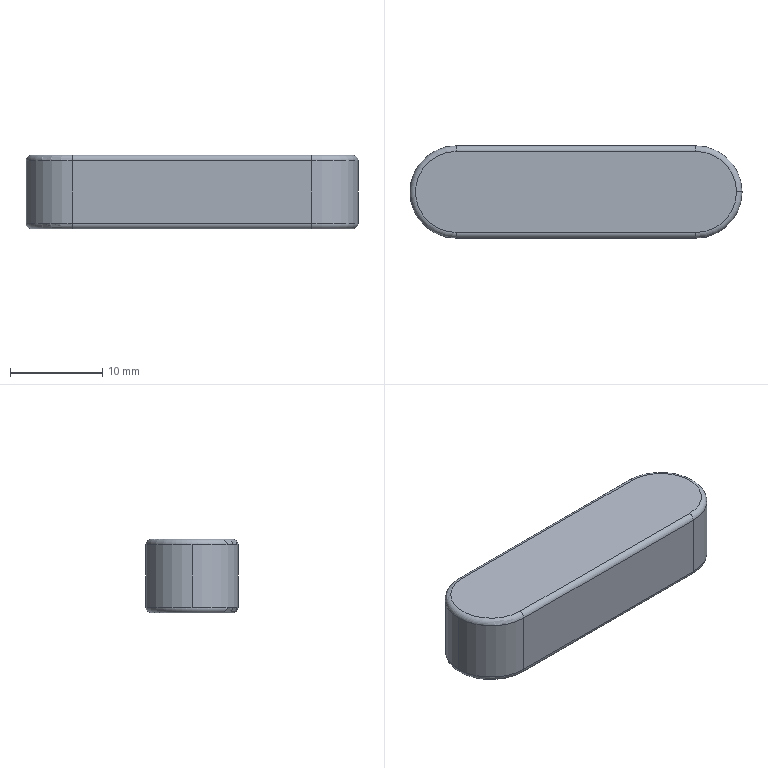Part | SolidWorks | features Extrusion 1, Fillet 1 | 1 solid | 17 faces | box 36 x 10 x 8 mm | volume 2696 mm3 | cylinder 7 | torus 6 | plane 4 | commonest cylinder face diameters 1.2 x4 10 x3
STEP:
#1=CARTESIAN_POINT('',(17.4,0.,0.));
#2=VERTEX_POINT('',#1);
#3=CARTESIAN_POINT('',(13.,-4.4,0.));
#4=VERTEX_POINT('',#3);
#5=CARTESIAN_POINT('',(13.,0.,0.));
#6=DIRECTION('',(0.,0.,-1.));
#7=DIRECTION('',(1.,0.,0.));
#8=AXIS2_PLACEMENT_3D('',#5,#6,#7);
#9=CIRCLE('',#8,4.4);
#10=EDGE_CURVE('',#2,#4,#9,.T.);
#11=ORIENTED_EDGE('',*,*,#10,.F.);
#12=CARTESIAN_POINT('',(18.,0.,0.6));
#13=VERTEX_POINT('',#12);
#14=CARTESIAN_POINT('',(17.4,0.,0.6));
#15=DIRECTION('',(0.,-1.,0.));
#16=DIRECTION('',(0.,0.,-1.));
#17=AXIS2_PLACEMENT_3D('',#14,#15,#16);
#18=CIRCLE('',#17,0.6);
#19=EDGE_CURVE('',#2,#13,#18,.T.);
#20=ORIENTED_EDGE('',*,*,#19,.T.);
#21=CARTESIAN_POINT('',(13.,-5.,0.6));
#22=VERTEX_POINT('',#21);
#23=CARTESIAN_POINT('',(13.,0.,0.6));
#24=DIRECTION('',(0.,0.,1.));
#25=DIRECTION('',(1.,0.,0.));
#26=AXIS2_PLACEMENT_3D('',#23,#24,#25);
#27=CIRCLE('',#26,5.);
#28=EDGE_CURVE('',#22,#13,#27,.T.);
#29=ORIENTED_EDGE('',*,*,#28,.F.);
#30=CARTESIAN_POINT('',(13.,-4.4,0.6));
#31=DIRECTION('',(1.,0.,0.));
#32=DIRECTION('',(0.,0.,-1.));
#33=AXIS2_PLACEMENT_3D('',#30,#31,#32);
#34=CIRCLE('',#33,0.6);
#35=EDGE_CURVE('',#22,#4,#34,.T.);
#36=ORIENTED_EDGE('',*,*,#35,.T.);
#37=EDGE_LOOP('',(#11,#20,#29,#36));
#38=FACE_OUTER_BOUND('',#37,.T.);
#39=CARTESIAN_POINT('',(13.,0.,0.6));
#40=DIRECTION('',(0.,0.,1.));
#41=DIRECTION('',(1.,0.,0.));
#42=AXIS2_PLACEMENT_3D('',#39,#40,#41);
#43=TOROIDAL_SURFACE('',#42,4.4,0.6);
#44=ADVANCED_FACE('',(#38),#43,.T.);
#45=CARTESIAN_POINT('',(18.,0.,7.4));
#46=VERTEX_POINT('',#45);
#47=CARTESIAN_POINT('',(13.,-5.,7.4));
#48=VERTEX_POINT('',#47);
#49=CARTESIAN_POINT('',(13.,0.,7.4));
#50=DIRECTION('',(0.,0.,-1.));
#51=DIRECTION('',(1.,0.,0.));
#52=AXIS2_PLACEMENT_3D('',#49,#50,#51);
#53=CIRCLE('',#52,5.);
#54=EDGE_CURVE('',#46,#48,#53,.T.);
#55=ORIENTED_EDGE('',*,*,#54,.F.);
#56=CARTESIAN_POINT('',(17.4,0.,8.));
#57=VERTEX_POINT('',#56);
#58=CARTESIAN_POINT('',(17.4,0.,7.4));
#59=DIRECTION('',(0.,-1.,0.));
#60=DIRECTION('',(0.,0.,-1.));
#61=AXIS2_PLACEMENT_3D('',#58,#59,#60);
#62=CIRCLE('',#61,0.6);
#63=EDGE_CURVE('',#46,#57,#62,.T.);
#64=ORIENTED_EDGE('',*,*,#63,.T.);
#65=CARTESIAN_POINT('',(13.,-4.4,8.));
#66=VERTEX_POINT('',#65);
#67=CARTESIAN_POINT('',(13.,0.,8.));
#68=DIRECTION('',(0.,0.,1.));
#69=DIRECTION('',(1.,0.,0.));
#70=AXIS2_PLACEMENT_3D('',#67,#68,#69);
#71=CIRCLE('',#70,4.4);
#72=EDGE_CURVE('',#66,#57,#71,.T.);
#73=ORIENTED_EDGE('',*,*,#72,.F.);
#74=CARTESIAN_POINT('',(13.,-4.4,7.4));
#75=DIRECTION('',(1.,0.,0.));
#76=DIRECTION('',(0.,0.,-1.));
#77=AXIS2_PLACEMENT_3D('',#74,#75,#76);
#78=CIRCLE('',#77,0.6);
#79=EDGE_CURVE('',#66,#48,#78,.T.);
#80=ORIENTED_EDGE('',*,*,#79,.T.);
#81=EDGE_LOOP('',(#55,#64,#73,#80));
#82=FACE_OUTER_BOUND('',#81,.T.);
#83=CARTESIAN_POINT('',(13.,0.,7.4));
#84=DIRECTION('',(0.,0.,1.));
#85=DIRECTION('',(1.,0.,0.));
#86=AXIS2_PLACEMENT_3D('',#83,#84,#85);
#87=TOROIDAL_SURFACE('',#86,4.4,0.6);
#88=ADVANCED_FACE('',(#82),#87,.T.);
#89=CARTESIAN_POINT('',(-13.,-5.,7.4));
#90=VERTEX_POINT('',#89);
#91=CARTESIAN_POINT('',(-18.,0.,7.4));
#92=VERTEX_POINT('',#91);
#93=CARTESIAN_POINT('',(-13.,0.,7.4));
#94=DIRECTION('',(0.,0.,-1.));
#95=DIRECTION('',(1.,0.,0.));
#96=AXIS2_PLACEMENT_3D('',#93,#94,#95);
#97=CIRCLE('',#96,5.);
#98=EDGE_CURVE('',#90,#92,#97,.T.);
#99=ORIENTED_EDGE('',*,*,#98,.T.);
#100=CARTESIAN_POINT('',(-18.,0.,0.6));
#101=VERTEX_POINT('',#100);
#102=CARTESIAN_POINT('',(-18.,0.,8.));
#103=DIRECTION('',(0.,0.,-1.));
#104=VECTOR('',#103,1000.);
#105=LINE('',#102,#104);
#106=EDGE_CURVE('',#92,#101,#105,.T.);
#107=ORIENTED_EDGE('',*,*,#106,.T.);
#108=CARTESIAN_POINT('',(-13.,-5.,0.6));
#109=VERTEX_POINT('',#108);
#110=CARTESIAN_POINT('',(-13.,0.,0.6));
#111=DIRECTION('',(0.,0.,1.));
#112=DIRECTION('',(1.,0.,0.));
#113=AXIS2_PLACEMENT_3D('',#110,#111,#112);
#114=CIRCLE('',#113,5.);
#115=EDGE_CURVE('',#101,#109,#114,.T.);
#116=ORIENTED_EDGE('',*,*,#115,.T.);
#117=CARTESIAN_POINT('',(-13.,-5.,8.));
#118=DIRECTION('',(0.,0.,-1.));
#119=VECTOR('',#118,1000.);
#120=LINE('',#117,#119);
#121=EDGE_CURVE('',#90,#109,#120,.T.);
#122=ORIENTED_EDGE('',*,*,#121,.F.);
#123=EDGE_LOOP('',(#99,#107,#116,#122));
#124=FACE_OUTER_BOUND('',#123,.T.);
#125=CARTESIAN_POINT('',(-13.,0.,8.));
#126=DIRECTION('',(0.,0.,-1.));
#127=DIRECTION('',(-1.,0.,0.));
#128=AXIS2_PLACEMENT_3D('',#125,#126,#127);
#129=CYLINDRICAL_SURFACE('',#128,5.);
#130=ADVANCED_FACE('',(#124),#129,.T.);
#131=ORIENTED_EDGE('',*,*,#106,.F.);
#132=CARTESIAN_POINT('',(-13.,5.,7.4));
#133=VERTEX_POINT('',#132);
#134=CARTESIAN_POINT('',(-13.,0.,7.4));
#135=DIRECTION('',(0.,0.,-1.));
#136=DIRECTION('',(1.,0.,0.));
#137=AXIS2_PLACEMENT_3D('',#134,#135,#136);
#138=CIRCLE('',#137,5.);
#139=EDGE_CURVE('',#92,#133,#138,.T.);
#140=ORIENTED_EDGE('',*,*,#139,.T.);
#141=CARTESIAN_POINT('',(-13.,5.,0.6));
#142=VERTEX_POINT('',#141);
#143=CARTESIAN_POINT('',(-13.,5.,8.));
#144=DIRECTION('',(0.,0.,-1.));
#145=VECTOR('',#144,1000.);
#146=LINE('',#143,#145);
#147=EDGE_CURVE('',#133,#142,#146,.T.);
#148=ORIENTED_EDGE('',*,*,#147,.T.);
#149=CARTESIAN_POINT('',(-13.,0.,0.6));
#150=DIRECTION('',(0.,0.,1.));
#151=DIRECTION('',(1.,0.,0.));
#152=AXIS2_PLACEMENT_3D('',#149,#150,#151);
#153=CIRCLE('',#152,5.);
#154=EDGE_CURVE('',#142,#101,#153,.T.);
#155=ORIENTED_EDGE('',*,*,#154,.T.);
#156=EDGE_LOOP('',(#131,#140,#148,#155));
#157=FACE_OUTER_BOUND('',#156,.T.);
#158=CARTESIAN_POINT('',(-13.,0.,8.));
#159=DIRECTION('',(0.,0.,-1.));
#160=DIRECTION('',(-1.,0.,0.));
#161=AXIS2_PLACEMENT_3D('',#158,#159,#160);
#162=CYLINDRICAL_SURFACE('',#161,5.);
#163=ADVANCED_FACE('',(#157),#162,.T.);
#164=CARTESIAN_POINT('',(13.,-5.,8.));
#165=DIRECTION('',(0.,0.,-1.));
#166=VECTOR('',#165,1000.);
#167=LINE('',#164,#166);
#168=EDGE_CURVE('',#48,#22,#167,.T.);
#169=ORIENTED_EDGE('',*,*,#168,.F.);
#170=CARTESIAN_POINT('',(-13.,-5.,7.4));
#171=DIRECTION('',(-1.,0.,0.));
#172=VECTOR('',#171,1000.);
#173=LINE('',#170,#172);
#174=EDGE_CURVE('',#48,#90,#173,.T.);
#175=ORIENTED_EDGE('',*,*,#174,.T.);
#176=ORIENTED_EDGE('',*,*,#121,.T.);
#177=CARTESIAN_POINT('',(-13.,-5.,0.6));
#178=DIRECTION('',(1.,0.,0.));
#179=VECTOR('',#178,1000.);
#180=LINE('',#177,#179);
#181=EDGE_CURVE('',#109,#22,#180,.T.);
#182=ORIENTED_EDGE('',*,*,#181,.T.);
#183=EDGE_LOOP('',(#169,#175,#176,#182));
#184=FACE_OUTER_BOUND('',#183,.T.);
#185=CARTESIAN_POINT('',(-13.,-5.,8.));
#186=DIRECTION('',(0.,1.,0.));
#187=DIRECTION('',(-1.,0.,0.));
#188=AXIS2_PLACEMENT_3D('',#185,#186,#187);
#189=PLANE('',#188);
#190=ADVANCED_FACE('',(#184),#189,.F.);
#191=CARTESIAN_POINT('',(13.,5.,7.4));
#192=VERTEX_POINT('',#191);
#193=CARTESIAN_POINT('',(13.,5.,0.6));
#194=VERTEX_POINT('',#193);
#195=CARTESIAN_POINT('',(13.,5.,8.));
#196=DIRECTION('',(0.,0.,-1.));
#197=VECTOR('',#196,1000.);
#198=LINE('',#195,#197);
#199=EDGE_CURVE('',#192,#194,#198,.T.);
#200=ORIENTED_EDGE('',*,*,#199,.F.);
#201=CARTESIAN_POINT('',(13.,0.,7.4));
#202=DIRECTION('',(0.,0.,-1.));
#203=DIRECTION('',(1.,0.,0.));
#204=AXIS2_PLACEMENT_3D('',#201,#202,#203);
#205=CIRCLE('',#204,5.);
#206=EDGE_CURVE('',#192,#46,#205,.T.);
#207=ORIENTED_EDGE('',*,*,#206,.T.);
#208=ORIENTED_EDGE('',*,*,#54,.T.);
#209=ORIENTED_EDGE('',*,*,#168,.T.);
#210=ORIENTED_EDGE('',*,*,#28,.T.);
#211=CARTESIAN_POINT('',(13.,0.,0.6));
#212=DIRECTION('',(0.,0.,1.));
#213=DIRECTION('',(1.,0.,0.));
#214=AXIS2_PLACEMENT_3D('',#211,#212,#213);
#215=CIRCLE('',#214,5.);
#216=EDGE_CURVE('',#13,#194,#215,.T.);
#217=ORIENTED_EDGE('',*,*,#216,.T.);
#218=EDGE_LOOP('',(#200,#207,#208,#209,#210,#217));
#219=FACE_OUTER_BOUND('',#218,.T.);
#220=CARTESIAN_POINT('',(13.,0.,8.));
#221=DIRECTION('',(0.,0.,-1.));
#222=DIRECTION('',(-1.,0.,0.));
#223=AXIS2_PLACEMENT_3D('',#220,#221,#222);
#224=CYLINDRICAL_SURFACE('',#223,5.);
#225=ADVANCED_FACE('',(#219),#224,.T.);
#226=ORIENTED_EDGE('',*,*,#147,.F.);
#227=CARTESIAN_POINT('',(13.,5.,7.4));
#228=DIRECTION('',(1.,0.,0.));
#229=VECTOR('',#228,1000.);
#230=LINE('',#227,#229);
#231=EDGE_CURVE('',#133,#192,#230,.T.);
#232=ORIENTED_EDGE('',*,*,#231,.T.);
#233=ORIENTED_EDGE('',*,*,#199,.T.);
#234=CARTESIAN_POINT('',(-13.,5.,0.6));
#235=DIRECTION('',(-1.,0.,0.));
#236=VECTOR('',#235,1000.);
#237=LINE('',#234,#236);
#238=EDGE_CURVE('',#194,#142,#237,.T.);
#239=ORIENTED_EDGE('',*,*,#238,.T.);
#240=EDGE_LOOP('',(#226,#232,#233,#239));
#241=FACE_OUTER_BOUND('',#240,.T.);
#242=CARTESIAN_POINT('',(-13.,5.,8.));
#243=DIRECTION('',(0.,-1.,0.));
#244=DIRECTION('',(1.,0.,0.));
#245=AXIS2_PLACEMENT_3D('',#242,#243,#244);
#246=PLANE('',#245);
#247=ADVANCED_FACE('',(#241),#246,.F.);
#248=CARTESIAN_POINT('',(-13.,-4.4,8.));
#249=VERTEX_POINT('',#248);
#250=CARTESIAN_POINT('',(13.,-4.4,8.));
#251=DIRECTION('',(1.,0.,0.));
#252=VECTOR('',#251,1000.);
#253=LINE('',#250,#252);
#254=EDGE_CURVE('',#249,#66,#253,.T.);
#255=ORIENTED_EDGE('',*,*,#254,.T.);
#256=ORIENTED_EDGE('',*,*,#72,.T.);
#257=CARTESIAN_POINT('',(13.,4.4,8.));
#258=VERTEX_POINT('',#257);
#259=CARTESIAN_POINT('',(13.,0.,8.));
#260=DIRECTION('',(0.,0.,1.));
#261=DIRECTION('',(1.,0.,0.));
#262=AXIS2_PLACEMENT_3D('',#259,#260,#261);
#263=CIRCLE('',#262,4.4);
#264=EDGE_CURVE('',#57,#258,#263,.T.);
#265=ORIENTED_EDGE('',*,*,#264,.T.);
#266=CARTESIAN_POINT('',(-13.,4.4,8.));
#267=VERTEX_POINT('',#266);
#268=CARTESIAN_POINT('',(-13.,4.4,8.));
#269=DIRECTION('',(-1.,0.,0.));
#270=VECTOR('',#269,1000.);
#271=LINE('',#268,#270);
#272=EDGE_CURVE('',#258,#267,#271,.T.);
#273=ORIENTED_EDGE('',*,*,#272,.T.);
#274=CARTESIAN_POINT('',(-13.,0.,8.));
#275=DIRECTION('',(0.,0.,1.));
#276=DIRECTION('',(1.,0.,0.));
#277=AXIS2_PLACEMENT_3D('',#274,#275,#276);
#278=CIRCLE('',#277,4.4);
#279=EDGE_CURVE('',#267,#249,#278,.T.);
#280=ORIENTED_EDGE('',*,*,#279,.T.);
#281=EDGE_LOOP('',(#255,#256,#265,#273,#280));
#282=FACE_OUTER_BOUND('',#281,.T.);
#283=CARTESIAN_POINT('',(-13.,0.,8.));
#284=DIRECTION('',(0.,0.,1.));
#285=DIRECTION('',(1.,0.,0.));
#286=AXIS2_PLACEMENT_3D('',#283,#284,#285);
#287=PLANE('',#286);
#288=ADVANCED_FACE('',(#282),#287,.T.);
#289=CARTESIAN_POINT('',(-13.,4.4,0.));
#290=VERTEX_POINT('',#289);
#291=CARTESIAN_POINT('',(13.,4.4,0.));
#292=VERTEX_POINT('',#291);
#293=CARTESIAN_POINT('',(-13.,4.4,0.));
#294=DIRECTION('',(1.,0.,0.));
#295=VECTOR('',#294,1000.);
#296=LINE('',#293,#295);
#297=EDGE_CURVE('',#290,#292,#296,.T.);
#298=ORIENTED_EDGE('',*,*,#297,.T.);
#299=CARTESIAN_POINT('',(13.,0.,0.));
#300=DIRECTION('',(0.,0.,-1.));
#301=DIRECTION('',(1.,0.,0.));
#302=AXIS2_PLACEMENT_3D('',#299,#300,#301);
#303=CIRCLE('',#302,4.4);
#304=EDGE_CURVE('',#292,#2,#303,.T.);
#305=ORIENTED_EDGE('',*,*,#304,.T.);
#306=ORIENTED_EDGE('',*,*,#10,.T.);
#307=CARTESIAN_POINT('',(-13.,-4.4,0.));
#308=VERTEX_POINT('',#307);
#309=CARTESIAN_POINT('',(-13.,-4.4,0.));
#310=DIRECTION('',(-1.,0.,0.));
#311=VECTOR('',#310,1000.);
#312=LINE('',#309,#311);
#313=EDGE_CURVE('',#4,#308,#312,.T.);
#314=ORIENTED_EDGE('',*,*,#313,.T.);
#315=CARTESIAN_POINT('',(-13.,0.,0.));
#316=DIRECTION('',(0.,0.,-1.));
#317=DIRECTION('',(1.,0.,0.));
#318=AXIS2_PLACEMENT_3D('',#315,#316,#317);
#319=CIRCLE('',#318,4.4);
#320=EDGE_CURVE('',#308,#290,#319,.T.);
#321=ORIENTED_EDGE('',*,*,#320,.T.);
#322=EDGE_LOOP('',(#298,#305,#306,#314,#321));
#323=FACE_OUTER_BOUND('',#322,.T.);
#324=CARTESIAN_POINT('',(-13.,0.,0.));
#325=DIRECTION('',(0.,0.,1.));
#326=DIRECTION('',(1.,0.,0.));
#327=AXIS2_PLACEMENT_3D('',#324,#325,#326);
#328=PLANE('',#327);
#329=ADVANCED_FACE('',(#323),#328,.F.);
#330=CARTESIAN_POINT('',(-13.,4.4,7.4));
#331=DIRECTION('',(1.,0.,0.));
#332=DIRECTION('',(0.,0.,-1.));
#333=AXIS2_PLACEMENT_3D('',#330,#331,#332);
#334=CIRCLE('',#333,0.6);
#335=EDGE_CURVE('',#133,#267,#334,.T.);
#336=ORIENTED_EDGE('',*,*,#335,.F.);
#337=ORIENTED_EDGE('',*,*,#139,.F.);
#338=ORIENTED_EDGE('',*,*,#98,.F.);
#339=CARTESIAN_POINT('',(-13.,-4.4,7.4));
#340=DIRECTION('',(1.,0.,0.));
#341=DIRECTION('',(0.,0.,-1.));
#342=AXIS2_PLACEMENT_3D('',#339,#340,#341);
#343=CIRCLE('',#342,0.6);
#344=EDGE_CURVE('',#249,#90,#343,.T.);
#345=ORIENTED_EDGE('',*,*,#344,.F.);
#346=ORIENTED_EDGE('',*,*,#279,.F.);
#347=EDGE_LOOP('',(#336,#337,#338,#345,#346));
#348=FACE_OUTER_BOUND('',#347,.T.);
#349=CARTESIAN_POINT('',(-13.,0.,7.4));
#350=DIRECTION('',(0.,0.,1.));
#351=DIRECTION('',(1.,0.,0.));
#352=AXIS2_PLACEMENT_3D('',#349,#350,#351);
#353=TOROIDAL_SURFACE('',#352,4.4,0.6);
#354=ADVANCED_FACE('',(#348),#353,.T.);
#355=ORIENTED_EDGE('',*,*,#344,.T.);
#356=ORIENTED_EDGE('',*,*,#174,.F.);
#357=ORIENTED_EDGE('',*,*,#79,.F.);
#358=ORIENTED_EDGE('',*,*,#254,.F.);
#359=EDGE_LOOP('',(#355,#356,#357,#358));
#360=FACE_OUTER_BOUND('',#359,.T.);
#361=CARTESIAN_POINT('',(-13.,-4.4,7.4));
#362=DIRECTION('',(-1.,0.,0.));
#363=DIRECTION('',(0.,-1.,0.));
#364=AXIS2_PLACEMENT_3D('',#361,#362,#363);
#365=CYLINDRICAL_SURFACE('',#364,0.6);
#366=ADVANCED_FACE('',(#360),#365,.T.);
#367=ORIENTED_EDGE('',*,*,#335,.T.);
#368=ORIENTED_EDGE('',*,*,#272,.F.);
#369=CARTESIAN_POINT('',(13.,4.4,7.4));
#370=DIRECTION('',(1.,0.,0.));
#371=DIRECTION('',(0.,0.,-1.));
#372=AXIS2_PLACEMENT_3D('',#369,#370,#371);
#373=CIRCLE('',#372,0.6);
#374=EDGE_CURVE('',#192,#258,#373,.T.);
#375=ORIENTED_EDGE('',*,*,#374,.F.);
#376=ORIENTED_EDGE('',*,*,#231,.F.);
#377=EDGE_LOOP('',(#367,#368,#375,#376));
#378=FACE_OUTER_BOUND('',#377,.T.);
#379=CARTESIAN_POINT('',(-13.,4.4,7.4));
#380=DIRECTION('',(1.,0.,0.));
#381=DIRECTION('',(0.,1.,0.));
#382=AXIS2_PLACEMENT_3D('',#379,#380,#381);
#383=CYLINDRICAL_SURFACE('',#382,0.6);
#384=ADVANCED_FACE('',(#378),#383,.T.);
#385=ORIENTED_EDGE('',*,*,#63,.F.);
#386=ORIENTED_EDGE('',*,*,#206,.F.);
#387=ORIENTED_EDGE('',*,*,#374,.T.);
#388=ORIENTED_EDGE('',*,*,#264,.F.);
#389=EDGE_LOOP('',(#385,#386,#387,#388));
#390=FACE_OUTER_BOUND('',#389,.T.);
#391=CARTESIAN_POINT('',(13.,0.,7.4));
#392=DIRECTION('',(0.,0.,1.));
#393=DIRECTION('',(1.,0.,0.));
#394=AXIS2_PLACEMENT_3D('',#391,#392,#393);
#395=TOROIDAL_SURFACE('',#394,4.4,0.6);
#396=ADVANCED_FACE('',(#390),#395,.T.);
#397=CARTESIAN_POINT('',(-13.,4.4,0.6));
#398=DIRECTION('',(1.,0.,0.));
#399=DIRECTION('',(0.,0.,-1.));
#400=AXIS2_PLACEMENT_3D('',#397,#398,#399);
#401=CIRCLE('',#400,0.6);
#402=EDGE_CURVE('',#290,#142,#401,.T.);
#403=ORIENTED_EDGE('',*,*,#402,.F.);
#404=ORIENTED_EDGE('',*,*,#320,.F.);
#405=CARTESIAN_POINT('',(-13.,-4.4,0.6));
#406=DIRECTION('',(1.,0.,0.));
#407=DIRECTION('',(0.,0.,-1.));
#408=AXIS2_PLACEMENT_3D('',#405,#406,#407);
#409=CIRCLE('',#408,0.6);
#410=EDGE_CURVE('',#109,#308,#409,.T.);
#411=ORIENTED_EDGE('',*,*,#410,.F.);
#412=ORIENTED_EDGE('',*,*,#115,.F.);
#413=ORIENTED_EDGE('',*,*,#154,.F.);
#414=EDGE_LOOP('',(#403,#404,#411,#412,#413));
#415=FACE_OUTER_BOUND('',#414,.T.);
#416=CARTESIAN_POINT('',(-13.,0.,0.6));
#417=DIRECTION('',(0.,0.,1.));
#418=DIRECTION('',(1.,0.,0.));
#419=AXIS2_PLACEMENT_3D('',#416,#417,#418);
#420=TOROIDAL_SURFACE('',#419,4.4,0.6);
#421=ADVANCED_FACE('',(#415),#420,.T.);
#422=ORIENTED_EDGE('',*,*,#410,.T.);
#423=ORIENTED_EDGE('',*,*,#313,.F.);
#424=ORIENTED_EDGE('',*,*,#35,.F.);
#425=ORIENTED_EDGE('',*,*,#181,.F.);
#426=EDGE_LOOP('',(#422,#423,#424,#425));
#427=FACE_OUTER_BOUND('',#426,.T.);
#428=CARTESIAN_POINT('',(-13.,-4.4,0.6));
#429=DIRECTION('',(1.,0.,0.));
#430=DIRECTION('',(0.,1.,0.));
#431=AXIS2_PLACEMENT_3D('',#428,#429,#430);
#432=CYLINDRICAL_SURFACE('',#431,0.6);
#433=ADVANCED_FACE('',(#427),#432,.T.);
#434=ORIENTED_EDGE('',*,*,#402,.T.);
#435=ORIENTED_EDGE('',*,*,#238,.F.);
#436=CARTESIAN_POINT('',(13.,4.4,0.6));
#437=DIRECTION('',(1.,0.,0.));
#438=DIRECTION('',(0.,0.,-1.));
#439=AXIS2_PLACEMENT_3D('',#436,#437,#438);
#440=CIRCLE('',#439,0.6);
#441=EDGE_CURVE('',#292,#194,#440,.T.);
#442=ORIENTED_EDGE('',*,*,#441,.F.);
#443=ORIENTED_EDGE('',*,*,#297,.F.);
#444=EDGE_LOOP('',(#434,#435,#442,#443));
#445=FACE_OUTER_BOUND('',#444,.T.);
#446=CARTESIAN_POINT('',(-13.,4.4,0.6));
#447=DIRECTION('',(-1.,0.,0.));
#448=DIRECTION('',(0.,-1.,0.));
#449=AXIS2_PLACEMENT_3D('',#446,#447,#448);
#450=CYLINDRICAL_SURFACE('',#449,0.6);
#451=ADVANCED_FACE('',(#445),#450,.T.);
#452=ORIENTED_EDGE('',*,*,#19,.F.);
#453=ORIENTED_EDGE('',*,*,#304,.F.);
#454=ORIENTED_EDGE('',*,*,#441,.T.);
#455=ORIENTED_EDGE('',*,*,#216,.F.);
#456=EDGE_LOOP('',(#452,#453,#454,#455));
#457=FACE_OUTER_BOUND('',#456,.T.);
#458=CARTESIAN_POINT('',(13.,0.,0.6));
#459=DIRECTION('',(0.,0.,1.));
#460=DIRECTION('',(1.,0.,0.));
#461=AXIS2_PLACEMENT_3D('',#458,#459,#460);
#462=TOROIDAL_SURFACE('',#461,4.4,0.6);
#463=ADVANCED_FACE('',(#457),#462,.T.);
#464=CLOSED_SHELL('',(#44,#88,#130,#163,#190,#225,#247,#288,#329,#354,#366,#384,#396,#421,#433,#451,#463));
#465=MANIFOLD_SOLID_BREP('',#464);
#466=CARTESIAN_POINT('',(0.,0.,0.));
#467=DIRECTION('',(0.,0.,1.));
#468=DIRECTION('',(1.,0.,0.));
#469=AXIS2_PLACEMENT_3D('',#466,#467,#468);
#470=(LENGTH_UNIT()NAMED_UNIT(*)SI_UNIT(.MILLI.,.METRE.));
#471=UNCERTAINTY_MEASURE_WITH_UNIT(LENGTH_MEASURE(0.00001),#470,'','');
#472=(NAMED_UNIT(*)PLANE_ANGLE_UNIT()SI_UNIT($,.RADIAN.));
#473=(NAMED_UNIT(*)SI_UNIT($,.STERADIAN.)SOLID_ANGLE_UNIT());
#474=(GEOMETRIC_REPRESENTATION_CONTEXT(3)GLOBAL_UNCERTAINTY_ASSIGNED_CONTEXT((#471))GLOBAL_UNIT_ASSIGNED_CONTEXT((#470,#472,#473))REPRESENTATION_CONTEXT('',''));
#475=ADVANCED_BREP_SHAPE_REPRESENTATION('',(#465,#469),#474);